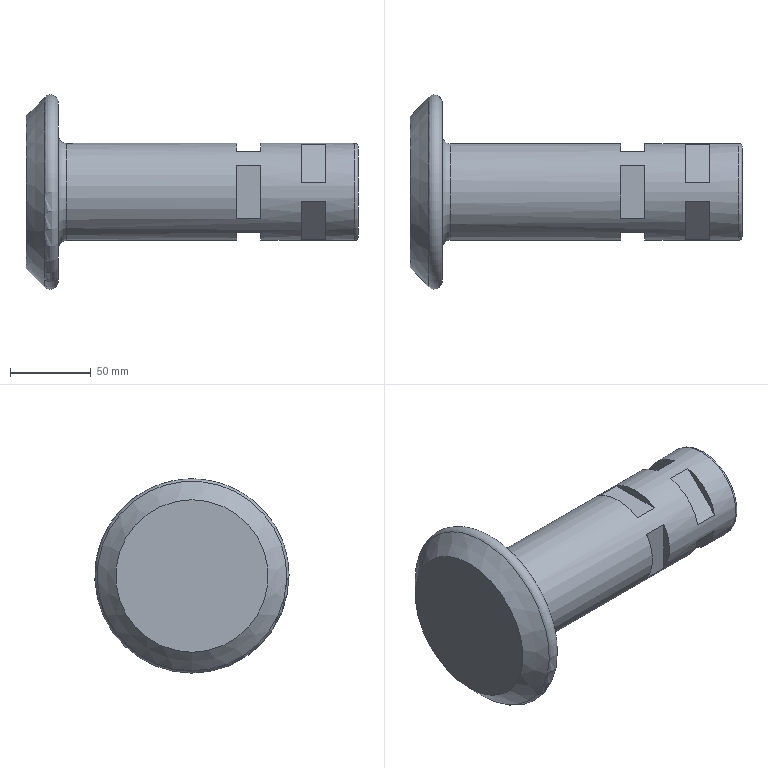Part | NX | features solid 2 | 1 solid | 32 faces | box 205 x 120 x 120 mm | volume 705223 mm3 | plane 27 | torus 3 | cylinder 1 | cone 1 | commonest cylinder face diameters 60 x1
STEP:
#1=CARTESIAN_POINT('',(-1050.,230.,-140.));
#2=VERTEX_POINT('',#1);
#3=CARTESIAN_POINT('',(-1050.,230.,-170.));
#4=DIRECTION('',(1.,0.,0.));
#5=DIRECTION('',(0.,0.,1.));
#6=AXIS2_PLACEMENT_3D('',#3,#4,#5);
#7=CIRCLE('',#6,30.);
#8=EDGE_CURVE('',#2,#2,#7,.F.);
#9=ORIENTED_EDGE('',*,*,#8,.F.);
#10=EDGE_LOOP('',(#9));
#11=FACE_BOUND('',#10,.T.);
#12=CARTESIAN_POINT('',(-890.,224.048,-140.596));
#13=VERTEX_POINT('',#12);
#14=CARTESIAN_POINT('',(-905.,224.048,-140.596));
#15=VERTEX_POINT('',#14);
#16=CARTESIAN_POINT('',(-1055.,224.048,-140.596));
#17=DIRECTION('',(1.,0.,0.));
#18=VECTOR('',#17,1000.);
#19=LINE('',#16,#18);
#20=EDGE_CURVE('',#13,#15,#19,.F.);
#21=ORIENTED_EDGE('',*,*,#20,.F.);
#22=CARTESIAN_POINT('',(-890.,200.596,-164.048));
#23=VERTEX_POINT('',#22);
#24=CARTESIAN_POINT('',(-890.,230.,-170.));
#25=DIRECTION('',(1.,0.,0.));
#26=DIRECTION('',(0.,0.,1.));
#27=AXIS2_PLACEMENT_3D('',#24,#25,#26);
#28=CIRCLE('',#27,30.);
#29=EDGE_CURVE('',#23,#13,#28,.F.);
#30=ORIENTED_EDGE('',*,*,#29,.F.);
#31=CARTESIAN_POINT('',(-905.,200.596,-164.048));
#32=VERTEX_POINT('',#31);
#33=CARTESIAN_POINT('',(-1055.,200.596,-164.048));
#34=DIRECTION('',(1.,0.,0.));
#35=VECTOR('',#34,1000.);
#36=LINE('',#33,#35);
#37=EDGE_CURVE('',#32,#23,#36,.T.);
#38=ORIENTED_EDGE('',*,*,#37,.F.);
#39=CARTESIAN_POINT('',(-905.,230.,-170.));
#40=DIRECTION('',(1.,0.,0.));
#41=DIRECTION('',(0.,0.,1.));
#42=AXIS2_PLACEMENT_3D('',#39,#40,#41);
#43=CIRCLE('',#42,30.);
#44=EDGE_CURVE('',#15,#32,#43,.T.);
#45=ORIENTED_EDGE('',*,*,#44,.F.);
#46=EDGE_LOOP('',(#21,#30,#38,#45));
#47=FACE_BOUND('',#46,.T.);
#48=CARTESIAN_POINT('',(-890.,200.596,-175.952));
#49=VERTEX_POINT('',#48);
#50=CARTESIAN_POINT('',(-905.,200.596,-175.952));
#51=VERTEX_POINT('',#50);
#52=CARTESIAN_POINT('',(-1055.,200.596,-175.952));
#53=DIRECTION('',(1.,0.,0.));
#54=VECTOR('',#53,1000.);
#55=LINE('',#52,#54);
#56=EDGE_CURVE('',#49,#51,#55,.F.);
#57=ORIENTED_EDGE('',*,*,#56,.F.);
#58=CARTESIAN_POINT('',(-890.,224.048,-199.404));
#59=VERTEX_POINT('',#58);
#60=CARTESIAN_POINT('',(-890.,230.,-170.));
#61=DIRECTION('',(1.,0.,0.));
#62=DIRECTION('',(0.,0.,1.));
#63=AXIS2_PLACEMENT_3D('',#60,#61,#62);
#64=CIRCLE('',#63,30.);
#65=EDGE_CURVE('',#59,#49,#64,.F.);
#66=ORIENTED_EDGE('',*,*,#65,.F.);
#67=CARTESIAN_POINT('',(-905.,224.048,-199.404));
#68=VERTEX_POINT('',#67);
#69=CARTESIAN_POINT('',(-1055.,224.048,-199.404));
#70=DIRECTION('',(1.,0.,0.));
#71=VECTOR('',#70,1000.);
#72=LINE('',#69,#71);
#73=EDGE_CURVE('',#68,#59,#72,.T.);
#74=ORIENTED_EDGE('',*,*,#73,.F.);
#75=CARTESIAN_POINT('',(-905.,230.,-170.));
#76=DIRECTION('',(1.,0.,0.));
#77=DIRECTION('',(0.,0.,1.));
#78=AXIS2_PLACEMENT_3D('',#75,#76,#77);
#79=CIRCLE('',#78,30.);
#80=EDGE_CURVE('',#51,#68,#79,.T.);
#81=ORIENTED_EDGE('',*,*,#80,.F.);
#82=EDGE_LOOP('',(#57,#66,#74,#81));
#83=FACE_BOUND('',#82,.T.);
#84=CARTESIAN_POINT('',(-930.,205.,-153.417));
#85=VERTEX_POINT('',#84);
#86=CARTESIAN_POINT('',(-945.,205.,-153.417));
#87=VERTEX_POINT('',#86);
#88=CARTESIAN_POINT('',(-1055.,205.,-153.417));
#89=DIRECTION('',(1.,0.,0.));
#90=VECTOR('',#89,1000.);
#91=LINE('',#88,#90);
#92=EDGE_CURVE('',#85,#87,#91,.F.);
#93=ORIENTED_EDGE('',*,*,#92,.F.);
#94=CARTESIAN_POINT('',(-930.,205.,-186.583));
#95=VERTEX_POINT('',#94);
#96=CARTESIAN_POINT('',(-930.,230.,-170.));
#97=DIRECTION('',(1.,0.,0.));
#98=DIRECTION('',(0.,0.,1.));
#99=AXIS2_PLACEMENT_3D('',#96,#97,#98);
#100=CIRCLE('',#99,30.);
#101=EDGE_CURVE('',#95,#85,#100,.F.);
#102=ORIENTED_EDGE('',*,*,#101,.F.);
#103=CARTESIAN_POINT('',(-945.,205.,-186.583));
#104=VERTEX_POINT('',#103);
#105=CARTESIAN_POINT('',(-1055.,205.,-186.583));
#106=DIRECTION('',(1.,0.,0.));
#107=VECTOR('',#106,1000.);
#108=LINE('',#105,#107);
#109=EDGE_CURVE('',#104,#95,#108,.T.);
#110=ORIENTED_EDGE('',*,*,#109,.F.);
#111=CARTESIAN_POINT('',(-945.,230.,-170.));
#112=DIRECTION('',(1.,0.,0.));
#113=DIRECTION('',(0.,0.,1.));
#114=AXIS2_PLACEMENT_3D('',#111,#112,#113);
#115=CIRCLE('',#114,30.);
#116=EDGE_CURVE('',#87,#104,#115,.T.);
#117=ORIENTED_EDGE('',*,*,#116,.F.);
#118=EDGE_LOOP('',(#93,#102,#110,#117));
#119=FACE_BOUND('',#118,.T.);
#120=CARTESIAN_POINT('',(-945.,246.583,-145.));
#121=VERTEX_POINT('',#120);
#122=CARTESIAN_POINT('',(-945.,213.417,-145.));
#123=VERTEX_POINT('',#122);
#124=CARTESIAN_POINT('',(-945.,230.,-170.));
#125=DIRECTION('',(1.,0.,0.));
#126=DIRECTION('',(0.,0.,1.));
#127=AXIS2_PLACEMENT_3D('',#124,#125,#126);
#128=CIRCLE('',#127,30.);
#129=EDGE_CURVE('',#121,#123,#128,.T.);
#130=ORIENTED_EDGE('',*,*,#129,.F.);
#131=CARTESIAN_POINT('',(-930.,246.583,-145.));
#132=VERTEX_POINT('',#131);
#133=CARTESIAN_POINT('',(-1055.,246.583,-145.));
#134=DIRECTION('',(1.,0.,0.));
#135=VECTOR('',#134,1000.);
#136=LINE('',#133,#135);
#137=EDGE_CURVE('',#132,#121,#136,.F.);
#138=ORIENTED_EDGE('',*,*,#137,.F.);
#139=CARTESIAN_POINT('',(-930.,213.417,-145.));
#140=VERTEX_POINT('',#139);
#141=CARTESIAN_POINT('',(-930.,230.,-170.));
#142=DIRECTION('',(1.,0.,0.));
#143=DIRECTION('',(0.,0.,1.));
#144=AXIS2_PLACEMENT_3D('',#141,#142,#143);
#145=CIRCLE('',#144,30.);
#146=EDGE_CURVE('',#140,#132,#145,.F.);
#147=ORIENTED_EDGE('',*,*,#146,.F.);
#148=CARTESIAN_POINT('',(-1055.,213.417,-145.));
#149=DIRECTION('',(1.,0.,0.));
#150=VECTOR('',#149,1000.);
#151=LINE('',#148,#150);
#152=EDGE_CURVE('',#123,#140,#151,.T.);
#153=ORIENTED_EDGE('',*,*,#152,.F.);
#154=EDGE_LOOP('',(#130,#138,#147,#153));
#155=FACE_BOUND('',#154,.T.);
#156=CARTESIAN_POINT('',(-872.,230.,-140.));
#157=VERTEX_POINT('',#156);
#158=CARTESIAN_POINT('',(-872.,230.,-170.));
#159=DIRECTION('',(1.,0.,0.));
#160=DIRECTION('',(0.,0.,1.));
#161=AXIS2_PLACEMENT_3D('',#158,#159,#160);
#162=CIRCLE('',#161,30.);
#163=EDGE_CURVE('',#157,#157,#162,.T.);
#164=ORIENTED_EDGE('',*,*,#163,.F.);
#165=EDGE_LOOP('',(#164));
#166=FACE_BOUND('',#165,.T.);
#167=CARTESIAN_POINT('',(-945.,246.583,-195.));
#168=VERTEX_POINT('',#167);
#169=CARTESIAN_POINT('',(-945.,213.417,-195.));
#170=VERTEX_POINT('',#169);
#171=CARTESIAN_POINT('',(-945.,230.,-170.));
#172=DIRECTION('',(1.,0.,0.));
#173=DIRECTION('',(0.,0.,1.));
#174=AXIS2_PLACEMENT_3D('',#171,#172,#173);
#175=CIRCLE('',#174,30.);
#176=EDGE_CURVE('',#168,#170,#175,.F.);
#177=ORIENTED_EDGE('',*,*,#176,.T.);
#178=CARTESIAN_POINT('',(-930.,213.417,-195.));
#179=VERTEX_POINT('',#178);
#180=CARTESIAN_POINT('',(-1055.,213.417,-195.));
#181=DIRECTION('',(1.,0.,0.));
#182=VECTOR('',#181,1000.);
#183=LINE('',#180,#182);
#184=EDGE_CURVE('',#170,#179,#183,.T.);
#185=ORIENTED_EDGE('',*,*,#184,.T.);
#186=CARTESIAN_POINT('',(-930.,246.583,-195.));
#187=VERTEX_POINT('',#186);
#188=CARTESIAN_POINT('',(-930.,230.,-170.));
#189=DIRECTION('',(1.,0.,0.));
#190=DIRECTION('',(0.,0.,1.));
#191=AXIS2_PLACEMENT_3D('',#188,#189,#190);
#192=CIRCLE('',#191,30.);
#193=EDGE_CURVE('',#179,#187,#192,.T.);
#194=ORIENTED_EDGE('',*,*,#193,.T.);
#195=CARTESIAN_POINT('',(-1055.,246.583,-195.));
#196=DIRECTION('',(1.,0.,0.));
#197=VECTOR('',#196,1000.);
#198=LINE('',#195,#197);
#199=EDGE_CURVE('',#187,#168,#198,.F.);
#200=ORIENTED_EDGE('',*,*,#199,.T.);
#201=EDGE_LOOP('',(#177,#185,#194,#200));
#202=FACE_BOUND('',#201,.T.);
#203=CARTESIAN_POINT('',(-945.,255.,-153.417));
#204=VERTEX_POINT('',#203);
#205=CARTESIAN_POINT('',(-945.,255.,-186.583));
#206=VERTEX_POINT('',#205);
#207=CARTESIAN_POINT('',(-945.,230.,-170.));
#208=DIRECTION('',(1.,0.,0.));
#209=DIRECTION('',(0.,0.,1.));
#210=AXIS2_PLACEMENT_3D('',#207,#208,#209);
#211=CIRCLE('',#210,30.);
#212=EDGE_CURVE('',#204,#206,#211,.F.);
#213=ORIENTED_EDGE('',*,*,#212,.T.);
#214=CARTESIAN_POINT('',(-930.,255.,-186.583));
#215=VERTEX_POINT('',#214);
#216=CARTESIAN_POINT('',(-1055.,255.,-186.583));
#217=DIRECTION('',(1.,0.,0.));
#218=VECTOR('',#217,1000.);
#219=LINE('',#216,#218);
#220=EDGE_CURVE('',#206,#215,#219,.T.);
#221=ORIENTED_EDGE('',*,*,#220,.T.);
#222=CARTESIAN_POINT('',(-930.,255.,-153.417));
#223=VERTEX_POINT('',#222);
#224=CARTESIAN_POINT('',(-930.,230.,-170.));
#225=DIRECTION('',(1.,0.,0.));
#226=DIRECTION('',(0.,0.,1.));
#227=AXIS2_PLACEMENT_3D('',#224,#225,#226);
#228=CIRCLE('',#227,30.);
#229=EDGE_CURVE('',#215,#223,#228,.T.);
#230=ORIENTED_EDGE('',*,*,#229,.T.);
#231=CARTESIAN_POINT('',(-1055.,255.,-153.417));
#232=DIRECTION('',(1.,0.,0.));
#233=VECTOR('',#232,1000.);
#234=LINE('',#231,#233);
#235=EDGE_CURVE('',#223,#204,#234,.F.);
#236=ORIENTED_EDGE('',*,*,#235,.T.);
#237=EDGE_LOOP('',(#213,#221,#230,#236));
#238=FACE_BOUND('',#237,.T.);
#239=CARTESIAN_POINT('',(-905.,235.952,-140.596));
#240=VERTEX_POINT('',#239);
#241=CARTESIAN_POINT('',(-905.,259.404,-164.048));
#242=VERTEX_POINT('',#241);
#243=CARTESIAN_POINT('',(-905.,230.,-170.));
#244=DIRECTION('',(1.,0.,0.));
#245=DIRECTION('',(0.,0.,1.));
#246=AXIS2_PLACEMENT_3D('',#243,#244,#245);
#247=CIRCLE('',#246,30.);
#248=EDGE_CURVE('',#240,#242,#247,.F.);
#249=ORIENTED_EDGE('',*,*,#248,.T.);
#250=CARTESIAN_POINT('',(-890.,259.404,-164.048));
#251=VERTEX_POINT('',#250);
#252=CARTESIAN_POINT('',(-1055.,259.404,-164.048));
#253=DIRECTION('',(1.,0.,0.));
#254=VECTOR('',#253,1000.);
#255=LINE('',#252,#254);
#256=EDGE_CURVE('',#242,#251,#255,.T.);
#257=ORIENTED_EDGE('',*,*,#256,.T.);
#258=CARTESIAN_POINT('',(-890.,235.952,-140.596));
#259=VERTEX_POINT('',#258);
#260=CARTESIAN_POINT('',(-890.,230.,-170.));
#261=DIRECTION('',(1.,0.,0.));
#262=DIRECTION('',(0.,0.,1.));
#263=AXIS2_PLACEMENT_3D('',#260,#261,#262);
#264=CIRCLE('',#263,30.);
#265=EDGE_CURVE('',#251,#259,#264,.T.);
#266=ORIENTED_EDGE('',*,*,#265,.T.);
#267=CARTESIAN_POINT('',(-1055.,235.952,-140.596));
#268=DIRECTION('',(1.,0.,0.));
#269=VECTOR('',#268,1000.);
#270=LINE('',#267,#269);
#271=EDGE_CURVE('',#259,#240,#270,.F.);
#272=ORIENTED_EDGE('',*,*,#271,.T.);
#273=EDGE_LOOP('',(#249,#257,#266,#272));
#274=FACE_BOUND('',#273,.T.);
#275=CARTESIAN_POINT('',(-905.,259.404,-175.952));
#276=VERTEX_POINT('',#275);
#277=CARTESIAN_POINT('',(-905.,235.952,-199.404));
#278=VERTEX_POINT('',#277);
#279=CARTESIAN_POINT('',(-905.,230.,-170.));
#280=DIRECTION('',(1.,0.,0.));
#281=DIRECTION('',(0.,0.,1.));
#282=AXIS2_PLACEMENT_3D('',#279,#280,#281);
#283=CIRCLE('',#282,30.);
#284=EDGE_CURVE('',#276,#278,#283,.F.);
#285=ORIENTED_EDGE('',*,*,#284,.T.);
#286=CARTESIAN_POINT('',(-890.,235.952,-199.404));
#287=VERTEX_POINT('',#286);
#288=CARTESIAN_POINT('',(-1055.,235.952,-199.404));
#289=DIRECTION('',(1.,0.,0.));
#290=VECTOR('',#289,1000.);
#291=LINE('',#288,#290);
#292=EDGE_CURVE('',#278,#287,#291,.T.);
#293=ORIENTED_EDGE('',*,*,#292,.T.);
#294=CARTESIAN_POINT('',(-890.,259.404,-175.952));
#295=VERTEX_POINT('',#294);
#296=CARTESIAN_POINT('',(-890.,230.,-170.));
#297=DIRECTION('',(1.,0.,0.));
#298=DIRECTION('',(0.,0.,1.));
#299=AXIS2_PLACEMENT_3D('',#296,#297,#298);
#300=CIRCLE('',#299,30.);
#301=EDGE_CURVE('',#287,#295,#300,.T.);
#302=ORIENTED_EDGE('',*,*,#301,.T.);
#303=CARTESIAN_POINT('',(-1055.,259.404,-175.952));
#304=DIRECTION('',(1.,0.,0.));
#305=VECTOR('',#304,1000.);
#306=LINE('',#303,#305);
#307=EDGE_CURVE('',#295,#276,#306,.F.);
#308=ORIENTED_EDGE('',*,*,#307,.T.);
#309=EDGE_LOOP('',(#285,#293,#302,#308));
#310=FACE_BOUND('',#309,.T.);
#311=CARTESIAN_POINT('',(-1055.,230.,-170.));
#312=DIRECTION('',(1.,0.,0.));
#313=DIRECTION('',(0.,0.,-1.));
#314=AXIS2_PLACEMENT_3D('',#311,#312,#313);
#315=CYLINDRICAL_SURFACE('',#314,30.);
#316=ADVANCED_FACE('',(#11,#47,#83,#119,#155,#166,#202,#238,#274,#310),#315,.T.);
#317=CARTESIAN_POINT('',(-870.,230.,-142.));
#318=VERTEX_POINT('',#317);
#319=CARTESIAN_POINT('',(-870.,230.,-170.));
#320=DIRECTION('',(1.,0.,0.));
#321=DIRECTION('',(0.,0.,1.));
#322=AXIS2_PLACEMENT_3D('',#319,#320,#321);
#323=CIRCLE('',#322,28.);
#324=EDGE_CURVE('',#318,#318,#323,.F.);
#325=ORIENTED_EDGE('',*,*,#324,.F.);
#326=EDGE_LOOP('',(#325));
#327=FACE_BOUND('',#326,.T.);
#328=CARTESIAN_POINT('',(-870.,200.,-170.));
#329=DIRECTION('',(-1.,0.,0.));
#330=DIRECTION('',(0.,0.,1.));
#331=AXIS2_PLACEMENT_3D('',#328,#329,#330);
#332=PLANE('',#331);
#333=ADVANCED_FACE('',(#327),#332,.F.);
#334=CARTESIAN_POINT('',(-1055.,230.,-135.));
#335=VERTEX_POINT('',#334);
#336=CARTESIAN_POINT('',(-1055.,230.,-170.));
#337=DIRECTION('',(1.,0.,0.));
#338=DIRECTION('',(0.,0.,1.));
#339=AXIS2_PLACEMENT_3D('',#336,#337,#338);
#340=CIRCLE('',#339,35.);
#341=EDGE_CURVE('',#335,#335,#340,.T.);
#342=ORIENTED_EDGE('',*,*,#341,.F.);
#343=EDGE_LOOP('',(#342));
#344=FACE_BOUND('',#343,.T.);
#345=CARTESIAN_POINT('',(-1055.,230.,-225.));
#346=VERTEX_POINT('',#345);
#347=CARTESIAN_POINT('',(-1055.,230.,-170.));
#348=DIRECTION('',(-1.,0.,0.));
#349=DIRECTION('',(0.,0.,-1.));
#350=AXIS2_PLACEMENT_3D('',#347,#348,#349);
#351=CIRCLE('',#350,55.);
#352=EDGE_CURVE('',#346,#346,#351,.T.);
#353=ORIENTED_EDGE('',*,*,#352,.F.);
#354=EDGE_LOOP('',(#353));
#355=FACE_BOUND('',#354,.T.);
#356=CARTESIAN_POINT('',(-1055.,175.,-170.));
#357=DIRECTION('',(-1.,0.,0.));
#358=DIRECTION('',(0.,0.,1.));
#359=AXIS2_PLACEMENT_3D('',#356,#357,#358);
#360=PLANE('',#359);
#361=ADVANCED_FACE('',(#344,#355),#360,.F.);
#362=CARTESIAN_POINT('',(-1063.536,230.,-228.536));
#363=VERTEX_POINT('',#362);
#364=CARTESIAN_POINT('',(-1063.536,230.,-170.));
#365=DIRECTION('',(-1.,0.,0.));
#366=DIRECTION('',(0.,0.,-1.));
#367=AXIS2_PLACEMENT_3D('',#364,#365,#366);
#368=CIRCLE('',#367,58.536);
#369=EDGE_CURVE('',#363,#363,#368,.T.);
#370=ORIENTED_EDGE('',*,*,#369,.T.);
#371=EDGE_LOOP('',(#370));
#372=FACE_BOUND('',#371,.T.);
#373=CARTESIAN_POINT('',(-1075.,230.,-217.071));
#374=VERTEX_POINT('',#373);
#375=CARTESIAN_POINT('',(-1075.,230.,-170.));
#376=DIRECTION('',(-1.,0.,0.));
#377=DIRECTION('',(0.,0.,-1.));
#378=AXIS2_PLACEMENT_3D('',#375,#376,#377);
#379=CIRCLE('',#378,47.071);
#380=EDGE_CURVE('',#374,#374,#379,.T.);
#381=ORIENTED_EDGE('',*,*,#380,.F.);
#382=EDGE_LOOP('',(#381));
#383=FACE_BOUND('',#382,.T.);
#384=CARTESIAN_POINT('',(-1075.,230.,-170.));
#385=DIRECTION('',(1.,0.,0.));
#386=DIRECTION('',(0.,0.,-1.));
#387=AXIS2_PLACEMENT_3D('',#384,#385,#386);
#388=CONICAL_SURFACE('',#387,47.071,0.7854);
#389=ADVANCED_FACE('',(#372,#383),#388,.T.);
#390=ORIENTED_EDGE('',*,*,#380,.T.);
#391=EDGE_LOOP('',(#390));
#392=FACE_BOUND('',#391,.T.);
#393=CARTESIAN_POINT('',(-1075.,230.,-170.));
#394=DIRECTION('',(1.,0.,0.));
#395=DIRECTION('',(0.,0.,-1.));
#396=AXIS2_PLACEMENT_3D('',#393,#394,#395);
#397=PLANE('',#396);
#398=ADVANCED_FACE('',(#392),#397,.F.);
#399=ORIENTED_EDGE('',*,*,#369,.F.);
#400=EDGE_LOOP('',(#399));
#401=FACE_BOUND('',#400,.T.);
#402=ORIENTED_EDGE('',*,*,#352,.T.);
#403=EDGE_LOOP('',(#402));
#404=FACE_BOUND('',#403,.T.);
#405=CARTESIAN_POINT('',(-1060.,230.,-170.));
#406=DIRECTION('',(1.,0.,0.));
#407=DIRECTION('',(0.,0.,-1.));
#408=AXIS2_PLACEMENT_3D('',#405,#406,#407);
#409=TOROIDAL_SURFACE('',#408,55.,5.);
#410=ADVANCED_FACE('',(#401,#404),#409,.T.);
#411=ORIENTED_EDGE('',*,*,#163,.T.);
#412=EDGE_LOOP('',(#411));
#413=FACE_BOUND('',#412,.T.);
#414=ORIENTED_EDGE('',*,*,#324,.T.);
#415=EDGE_LOOP('',(#414));
#416=FACE_BOUND('',#415,.T.);
#417=CARTESIAN_POINT('',(-872.,230.,-170.));
#418=DIRECTION('',(-1.,0.,0.));
#419=DIRECTION('',(0.,0.,1.));
#420=AXIS2_PLACEMENT_3D('',#417,#418,#419);
#421=TOROIDAL_SURFACE('',#420,28.,2.);
#422=ADVANCED_FACE('',(#413,#416),#421,.T.);
#423=CARTESIAN_POINT('',(-945.,255.,-195.));
#424=DIRECTION('',(0.,-1.,0.));
#425=VECTOR('',#424,1000.);
#426=LINE('',#423,#425);
#427=EDGE_CURVE('',#168,#170,#426,.T.);
#428=ORIENTED_EDGE('',*,*,#427,.T.);
#429=ORIENTED_EDGE('',*,*,#176,.F.);
#430=EDGE_LOOP('',(#428,#429));
#431=FACE_BOUND('',#430,.T.);
#432=CARTESIAN_POINT('',(-945.,255.,-170.));
#433=DIRECTION('',(-1.,0.,0.));
#434=DIRECTION('',(0.,-1.,0.));
#435=AXIS2_PLACEMENT_3D('',#432,#433,#434);
#436=PLANE('',#435);
#437=ADVANCED_FACE('',(#431),#436,.F.);
#438=CARTESIAN_POINT('',(-930.,255.,-195.));
#439=DIRECTION('',(0.,-1.,0.));
#440=VECTOR('',#439,1000.);
#441=LINE('',#438,#440);
#442=EDGE_CURVE('',#187,#179,#441,.T.);
#443=ORIENTED_EDGE('',*,*,#442,.F.);
#444=ORIENTED_EDGE('',*,*,#193,.F.);
#445=EDGE_LOOP('',(#443,#444));
#446=FACE_BOUND('',#445,.T.);
#447=CARTESIAN_POINT('',(-930.,255.,-170.));
#448=DIRECTION('',(-1.,0.,0.));
#449=DIRECTION('',(0.,-1.,0.));
#450=AXIS2_PLACEMENT_3D('',#447,#448,#449);
#451=PLANE('',#450);
#452=ADVANCED_FACE('',(#446),#451,.T.);
#453=ORIENTED_EDGE('',*,*,#184,.F.);
#454=ORIENTED_EDGE('',*,*,#427,.F.);
#455=ORIENTED_EDGE('',*,*,#199,.F.);
#456=ORIENTED_EDGE('',*,*,#442,.T.);
#457=EDGE_LOOP('',(#453,#454,#455,#456));
#458=FACE_BOUND('',#457,.T.);
#459=CARTESIAN_POINT('',(-945.,255.,-195.));
#460=DIRECTION('',(0.,0.,-1.));
#461=DIRECTION('',(0.,-1.,0.));
#462=AXIS2_PLACEMENT_3D('',#459,#460,#461);
#463=PLANE('',#462);
#464=ADVANCED_FACE('',(#458),#463,.T.);
#465=ORIENTED_EDGE('',*,*,#129,.T.);
#466=CARTESIAN_POINT('',(-945.,255.,-145.));
#467=DIRECTION('',(0.,-1.,0.));
#468=VECTOR('',#467,1000.);
#469=LINE('',#466,#468);
#470=EDGE_CURVE('',#121,#123,#469,.T.);
#471=ORIENTED_EDGE('',*,*,#470,.F.);
#472=EDGE_LOOP('',(#465,#471));
#473=FACE_BOUND('',#472,.T.);
#474=CARTESIAN_POINT('',(-945.,255.,-170.));
#475=DIRECTION('',(-1.,0.,0.));
#476=DIRECTION('',(0.,-1.,0.));
#477=AXIS2_PLACEMENT_3D('',#474,#475,#476);
#478=PLANE('',#477);
#479=ADVANCED_FACE('',(#473),#478,.F.);
#480=ORIENTED_EDGE('',*,*,#146,.T.);
#481=CARTESIAN_POINT('',(-930.,255.,-145.));
#482=DIRECTION('',(0.,-1.,0.));
#483=VECTOR('',#482,1000.);
#484=LINE('',#481,#483);
#485=EDGE_CURVE('',#132,#140,#484,.T.);
#486=ORIENTED_EDGE('',*,*,#485,.T.);
#487=EDGE_LOOP('',(#480,#486));
#488=FACE_BOUND('',#487,.T.);
#489=CARTESIAN_POINT('',(-930.,255.,-170.));
#490=DIRECTION('',(-1.,0.,0.));
#491=DIRECTION('',(0.,-1.,0.));
#492=AXIS2_PLACEMENT_3D('',#489,#490,#491);
#493=PLANE('',#492);
#494=ADVANCED_FACE('',(#488),#493,.T.);
#495=ORIENTED_EDGE('',*,*,#470,.T.);
#496=ORIENTED_EDGE('',*,*,#152,.T.);
#497=ORIENTED_EDGE('',*,*,#485,.F.);
#498=ORIENTED_EDGE('',*,*,#137,.T.);
#499=EDGE_LOOP('',(#495,#496,#497,#498));
#500=FACE_BOUND('',#499,.T.);
#501=CARTESIAN_POINT('',(-945.,255.,-145.));
#502=DIRECTION('',(0.,0.,-1.));
#503=DIRECTION('',(0.,-1.,0.));
#504=AXIS2_PLACEMENT_3D('',#501,#502,#503);
#505=PLANE('',#504);
#506=ADVANCED_FACE('',(#500),#505,.F.);
#507=CARTESIAN_POINT('',(-945.,255.,-145.));
#508=DIRECTION('',(0.,0.,-1.));
#509=VECTOR('',#508,1000.);
#510=LINE('',#507,#509);
#511=EDGE_CURVE('',#204,#206,#510,.T.);
#512=ORIENTED_EDGE('',*,*,#511,.T.);
#513=ORIENTED_EDGE('',*,*,#212,.F.);
#514=EDGE_LOOP('',(#512,#513));
#515=FACE_BOUND('',#514,.T.);
#516=CARTESIAN_POINT('',(-945.,230.,-145.));
#517=DIRECTION('',(-1.,0.,0.));
#518=DIRECTION('',(0.,0.,-1.));
#519=AXIS2_PLACEMENT_3D('',#516,#517,#518);
#520=PLANE('',#519);
#521=ADVANCED_FACE('',(#515),#520,.F.);
#522=CARTESIAN_POINT('',(-930.,255.,-145.));
#523=DIRECTION('',(0.,0.,-1.));
#524=VECTOR('',#523,1000.);
#525=LINE('',#522,#524);
#526=EDGE_CURVE('',#223,#215,#525,.T.);
#527=ORIENTED_EDGE('',*,*,#526,.F.);
#528=ORIENTED_EDGE('',*,*,#229,.F.);
#529=EDGE_LOOP('',(#527,#528));
#530=FACE_BOUND('',#529,.T.);
#531=CARTESIAN_POINT('',(-930.,230.,-145.));
#532=DIRECTION('',(-1.,0.,0.));
#533=DIRECTION('',(0.,0.,-1.));
#534=AXIS2_PLACEMENT_3D('',#531,#532,#533);
#535=PLANE('',#534);
#536=ADVANCED_FACE('',(#530),#535,.T.);
#537=ORIENTED_EDGE('',*,*,#220,.F.);
#538=ORIENTED_EDGE('',*,*,#511,.F.);
#539=ORIENTED_EDGE('',*,*,#235,.F.);
#540=ORIENTED_EDGE('',*,*,#526,.T.);
#541=EDGE_LOOP('',(#537,#538,#539,#540));
#542=FACE_BOUND('',#541,.T.);
#543=CARTESIAN_POINT('',(-945.,255.,-145.));
#544=DIRECTION('',(0.,1.,0.));
#545=DIRECTION('',(0.,0.,-1.));
#546=AXIS2_PLACEMENT_3D('',#543,#544,#545);
#547=PLANE('',#546);
#548=ADVANCED_FACE('',(#542),#547,.T.);
#549=CARTESIAN_POINT('',(-945.,205.,-145.));
#550=DIRECTION('',(0.,0.,-1.));
#551=VECTOR('',#550,1000.);
#552=LINE('',#549,#551);
#553=EDGE_CURVE('',#87,#104,#552,.T.);
#554=ORIENTED_EDGE('',*,*,#553,.F.);
#555=ORIENTED_EDGE('',*,*,#116,.T.);
#556=EDGE_LOOP('',(#554,#555));
#557=FACE_BOUND('',#556,.T.);
#558=CARTESIAN_POINT('',(-945.,230.,-145.));
#559=DIRECTION('',(-1.,0.,0.));
#560=DIRECTION('',(0.,0.,-1.));
#561=AXIS2_PLACEMENT_3D('',#558,#559,#560);
#562=PLANE('',#561);
#563=ADVANCED_FACE('',(#557),#562,.F.);
#564=CARTESIAN_POINT('',(-930.,205.,-145.));
#565=DIRECTION('',(0.,0.,-1.));
#566=VECTOR('',#565,1000.);
#567=LINE('',#564,#566);
#568=EDGE_CURVE('',#85,#95,#567,.T.);
#569=ORIENTED_EDGE('',*,*,#568,.T.);
#570=ORIENTED_EDGE('',*,*,#101,.T.);
#571=EDGE_LOOP('',(#569,#570));
#572=FACE_BOUND('',#571,.T.);
#573=CARTESIAN_POINT('',(-930.,230.,-145.));
#574=DIRECTION('',(-1.,0.,0.));
#575=DIRECTION('',(0.,0.,-1.));
#576=AXIS2_PLACEMENT_3D('',#573,#574,#575);
#577=PLANE('',#576);
#578=ADVANCED_FACE('',(#572),#577,.T.);
#579=ORIENTED_EDGE('',*,*,#553,.T.);
#580=ORIENTED_EDGE('',*,*,#109,.T.);
#581=ORIENTED_EDGE('',*,*,#568,.F.);
#582=ORIENTED_EDGE('',*,*,#92,.T.);
#583=EDGE_LOOP('',(#579,#580,#581,#582));
#584=FACE_BOUND('',#583,.T.);
#585=CARTESIAN_POINT('',(-945.,205.,-145.));
#586=DIRECTION('',(0.,1.,0.));
#587=DIRECTION('',(0.,0.,-1.));
#588=AXIS2_PLACEMENT_3D('',#585,#586,#587);
#589=PLANE('',#588);
#590=ADVANCED_FACE('',(#584),#589,.F.);
#591=CARTESIAN_POINT('',(-905.,194.645,-170.));
#592=DIRECTION('',(0.,0.7071,-0.7071));
#593=VECTOR('',#592,1000.);
#594=LINE('',#591,#593);
#595=EDGE_CURVE('',#51,#68,#594,.T.);
#596=ORIENTED_EDGE('',*,*,#595,.F.);
#597=ORIENTED_EDGE('',*,*,#80,.T.);
#598=EDGE_LOOP('',(#596,#597));
#599=FACE_BOUND('',#598,.T.);
#600=CARTESIAN_POINT('',(-905.,212.322,-152.322));
#601=DIRECTION('',(-1.,0.,0.));
#602=DIRECTION('',(0.,0.7071,-0.7071));
#603=AXIS2_PLACEMENT_3D('',#600,#601,#602);
#604=PLANE('',#603);
#605=ADVANCED_FACE('',(#599),#604,.F.);
#606=CARTESIAN_POINT('',(-890.,194.645,-170.));
#607=DIRECTION('',(0.,0.7071,-0.7071));
#608=VECTOR('',#607,1000.);
#609=LINE('',#606,#608);
#610=EDGE_CURVE('',#49,#59,#609,.T.);
#611=ORIENTED_EDGE('',*,*,#610,.T.);
#612=ORIENTED_EDGE('',*,*,#65,.T.);
#613=EDGE_LOOP('',(#611,#612));
#614=FACE_BOUND('',#613,.T.);
#615=CARTESIAN_POINT('',(-890.,212.322,-152.322));
#616=DIRECTION('',(-1.,0.,0.));
#617=DIRECTION('',(0.,0.7071,-0.7071));
#618=AXIS2_PLACEMENT_3D('',#615,#616,#617);
#619=PLANE('',#618);
#620=ADVANCED_FACE('',(#614),#619,.T.);
#621=ORIENTED_EDGE('',*,*,#595,.T.);
#622=ORIENTED_EDGE('',*,*,#73,.T.);
#623=ORIENTED_EDGE('',*,*,#610,.F.);
#624=ORIENTED_EDGE('',*,*,#56,.T.);
#625=EDGE_LOOP('',(#621,#622,#623,#624));
#626=FACE_BOUND('',#625,.T.);
#627=CARTESIAN_POINT('',(-905.,194.645,-170.));
#628=DIRECTION('',(0.,0.7071,0.7071));
#629=DIRECTION('',(0.,0.7071,-0.7071));
#630=AXIS2_PLACEMENT_3D('',#627,#628,#629);
#631=PLANE('',#630);
#632=ADVANCED_FACE('',(#626),#631,.F.);
#633=CARTESIAN_POINT('',(-905.,230.,-134.645));
#634=DIRECTION('',(0.,0.7071,-0.7071));
#635=VECTOR('',#634,1000.);
#636=LINE('',#633,#635);
#637=EDGE_CURVE('',#240,#242,#636,.T.);
#638=ORIENTED_EDGE('',*,*,#637,.T.);
#639=ORIENTED_EDGE('',*,*,#248,.F.);
#640=EDGE_LOOP('',(#638,#639));
#641=FACE_BOUND('',#640,.T.);
#642=CARTESIAN_POINT('',(-905.,212.322,-152.322));
#643=DIRECTION('',(-1.,0.,0.));
#644=DIRECTION('',(0.,0.7071,-0.7071));
#645=AXIS2_PLACEMENT_3D('',#642,#643,#644);
#646=PLANE('',#645);
#647=ADVANCED_FACE('',(#641),#646,.F.);
#648=CARTESIAN_POINT('',(-890.,230.,-134.645));
#649=DIRECTION('',(0.,0.7071,-0.7071));
#650=VECTOR('',#649,1000.);
#651=LINE('',#648,#650);
#652=EDGE_CURVE('',#259,#251,#651,.T.);
#653=ORIENTED_EDGE('',*,*,#652,.F.);
#654=ORIENTED_EDGE('',*,*,#265,.F.);
#655=EDGE_LOOP('',(#653,#654));
#656=FACE_BOUND('',#655,.T.);
#657=CARTESIAN_POINT('',(-890.,212.322,-152.322));
#658=DIRECTION('',(-1.,0.,0.));
#659=DIRECTION('',(0.,0.7071,-0.7071));
#660=AXIS2_PLACEMENT_3D('',#657,#658,#659);
#661=PLANE('',#660);
#662=ADVANCED_FACE('',(#656),#661,.T.);
#663=ORIENTED_EDGE('',*,*,#256,.F.);
#664=ORIENTED_EDGE('',*,*,#637,.F.);
#665=ORIENTED_EDGE('',*,*,#271,.F.);
#666=ORIENTED_EDGE('',*,*,#652,.T.);
#667=EDGE_LOOP('',(#663,#664,#665,#666));
#668=FACE_BOUND('',#667,.T.);
#669=CARTESIAN_POINT('',(-905.,230.,-134.645));
#670=DIRECTION('',(0.,0.7071,0.7071));
#671=DIRECTION('',(0.,0.7071,-0.7071));
#672=AXIS2_PLACEMENT_3D('',#669,#670,#671);
#673=PLANE('',#672);
#674=ADVANCED_FACE('',(#668),#673,.T.);
#675=CARTESIAN_POINT('',(-905.,265.355,-170.));
#676=DIRECTION('',(0.,-0.7071,-0.7071));
#677=VECTOR('',#676,1000.);
#678=LINE('',#675,#677);
#679=EDGE_CURVE('',#276,#278,#678,.T.);
#680=ORIENTED_EDGE('',*,*,#679,.T.);
#681=ORIENTED_EDGE('',*,*,#284,.F.);
#682=EDGE_LOOP('',(#680,#681));
#683=FACE_BOUND('',#682,.T.);
#684=CARTESIAN_POINT('',(-905.,247.678,-152.322));
#685=DIRECTION('',(-1.,0.,0.));
#686=DIRECTION('',(0.,-0.7071,-0.7071));
#687=AXIS2_PLACEMENT_3D('',#684,#685,#686);
#688=PLANE('',#687);
#689=ADVANCED_FACE('',(#683),#688,.F.);
#690=CARTESIAN_POINT('',(-890.,265.355,-170.));
#691=DIRECTION('',(0.,-0.7071,-0.7071));
#692=VECTOR('',#691,1000.);
#693=LINE('',#690,#692);
#694=EDGE_CURVE('',#295,#287,#693,.T.);
#695=ORIENTED_EDGE('',*,*,#694,.F.);
#696=ORIENTED_EDGE('',*,*,#301,.F.);
#697=EDGE_LOOP('',(#695,#696));
#698=FACE_BOUND('',#697,.T.);
#699=CARTESIAN_POINT('',(-890.,247.678,-152.322));
#700=DIRECTION('',(-1.,0.,0.));
#701=DIRECTION('',(0.,-0.7071,-0.7071));
#702=AXIS2_PLACEMENT_3D('',#699,#700,#701);
#703=PLANE('',#702);
#704=ADVANCED_FACE('',(#698),#703,.T.);
#705=ORIENTED_EDGE('',*,*,#292,.F.);
#706=ORIENTED_EDGE('',*,*,#679,.F.);
#707=ORIENTED_EDGE('',*,*,#307,.F.);
#708=ORIENTED_EDGE('',*,*,#694,.T.);
#709=EDGE_LOOP('',(#705,#706,#707,#708));
#710=FACE_BOUND('',#709,.T.);
#711=CARTESIAN_POINT('',(-905.,265.355,-170.));
#712=DIRECTION('',(0.,0.7071,-0.7071));
#713=DIRECTION('',(0.,-0.7071,-0.7071));
#714=AXIS2_PLACEMENT_3D('',#711,#712,#713);
#715=PLANE('',#714);
#716=ADVANCED_FACE('',(#710),#715,.T.);
#717=CARTESIAN_POINT('',(-905.,230.,-134.645));
#718=DIRECTION('',(0.,-0.7071,-0.7071));
#719=VECTOR('',#718,1000.);
#720=LINE('',#717,#719);
#721=EDGE_CURVE('',#15,#32,#720,.T.);
#722=ORIENTED_EDGE('',*,*,#721,.F.);
#723=ORIENTED_EDGE('',*,*,#44,.T.);
#724=EDGE_LOOP('',(#722,#723));
#725=FACE_BOUND('',#724,.T.);
#726=CARTESIAN_POINT('',(-905.,247.678,-152.322));
#727=DIRECTION('',(-1.,0.,0.));
#728=DIRECTION('',(0.,-0.7071,-0.7071));
#729=AXIS2_PLACEMENT_3D('',#726,#727,#728);
#730=PLANE('',#729);
#731=ADVANCED_FACE('',(#725),#730,.F.);
#732=CARTESIAN_POINT('',(-890.,230.,-134.645));
#733=DIRECTION('',(0.,-0.7071,-0.7071));
#734=VECTOR('',#733,1000.);
#735=LINE('',#732,#734);
#736=EDGE_CURVE('',#13,#23,#735,.T.);
#737=ORIENTED_EDGE('',*,*,#736,.T.);
#738=ORIENTED_EDGE('',*,*,#29,.T.);
#739=EDGE_LOOP('',(#737,#738));
#740=FACE_BOUND('',#739,.T.);
#741=CARTESIAN_POINT('',(-890.,247.678,-152.322));
#742=DIRECTION('',(-1.,0.,0.));
#743=DIRECTION('',(0.,-0.7071,-0.7071));
#744=AXIS2_PLACEMENT_3D('',#741,#742,#743);
#745=PLANE('',#744);
#746=ADVANCED_FACE('',(#740),#745,.T.);
#747=ORIENTED_EDGE('',*,*,#721,.T.);
#748=ORIENTED_EDGE('',*,*,#37,.T.);
#749=ORIENTED_EDGE('',*,*,#736,.F.);
#750=ORIENTED_EDGE('',*,*,#20,.T.);
#751=EDGE_LOOP('',(#747,#748,#749,#750));
#752=FACE_BOUND('',#751,.T.);
#753=CARTESIAN_POINT('',(-905.,230.,-134.645));
#754=DIRECTION('',(0.,0.7071,-0.7071));
#755=DIRECTION('',(0.,-0.7071,-0.7071));
#756=AXIS2_PLACEMENT_3D('',#753,#754,#755);
#757=PLANE('',#756);
#758=ADVANCED_FACE('',(#752),#757,.F.);
#759=ORIENTED_EDGE('',*,*,#341,.T.);
#760=EDGE_LOOP('',(#759));
#761=FACE_BOUND('',#760,.T.);
#762=ORIENTED_EDGE('',*,*,#8,.T.);
#763=EDGE_LOOP('',(#762));
#764=FACE_BOUND('',#763,.T.);
#765=CARTESIAN_POINT('',(-1050.,230.,-170.));
#766=DIRECTION('',(-1.,0.,0.));
#767=DIRECTION('',(0.,0.,1.));
#768=AXIS2_PLACEMENT_3D('',#765,#766,#767);
#769=TOROIDAL_SURFACE('',#768,35.,5.);
#770=ADVANCED_FACE('',(#761,#764),#769,.F.);
#771=CLOSED_SHELL('',(#316,#333,#361,#389,#398,#410,#422,#437,#452,#464,#479,#494,#506,#521,#536,#548,#563,#578,#590,#605,#620,#632,#647,#662,#674,#689,#704,#716,#731,#746,#758,#770));
#772=MANIFOLD_SOLID_BREP('',#771);
#773=(LENGTH_UNIT()NAMED_UNIT(*)SI_UNIT(.MILLI.,.METRE.));
#774=UNCERTAINTY_MEASURE_WITH_UNIT(LENGTH_MEASURE(0.00001),#773,'','');
#775=(NAMED_UNIT(*)PLANE_ANGLE_UNIT()SI_UNIT($,.RADIAN.));
#776=(NAMED_UNIT(*)SI_UNIT($,.STERADIAN.)SOLID_ANGLE_UNIT());
#777=(GEOMETRIC_REPRESENTATION_CONTEXT(3)GLOBAL_UNCERTAINTY_ASSIGNED_CONTEXT((#774))GLOBAL_UNIT_ASSIGNED_CONTEXT((#773,#775,#776))REPRESENTATION_CONTEXT('',''));
#778=ADVANCED_BREP_SHAPE_REPRESENTATION('',(#772),#777);